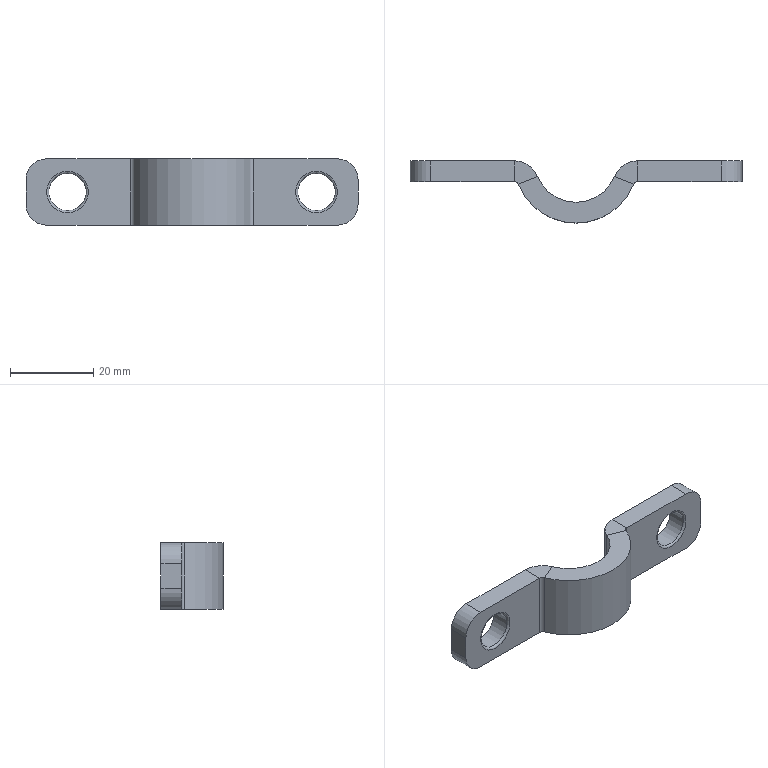Part | STEP file | PN_0010_default | 1 solid | 30 faces | box 80 x 15 x 16 mm | volume 6317 mm3 | plane 16 | cylinder 12 | torus 2 | commonest cylinder face diameters 10 x4 2 x2 9 x2 12 x2 20 x1 30 x1